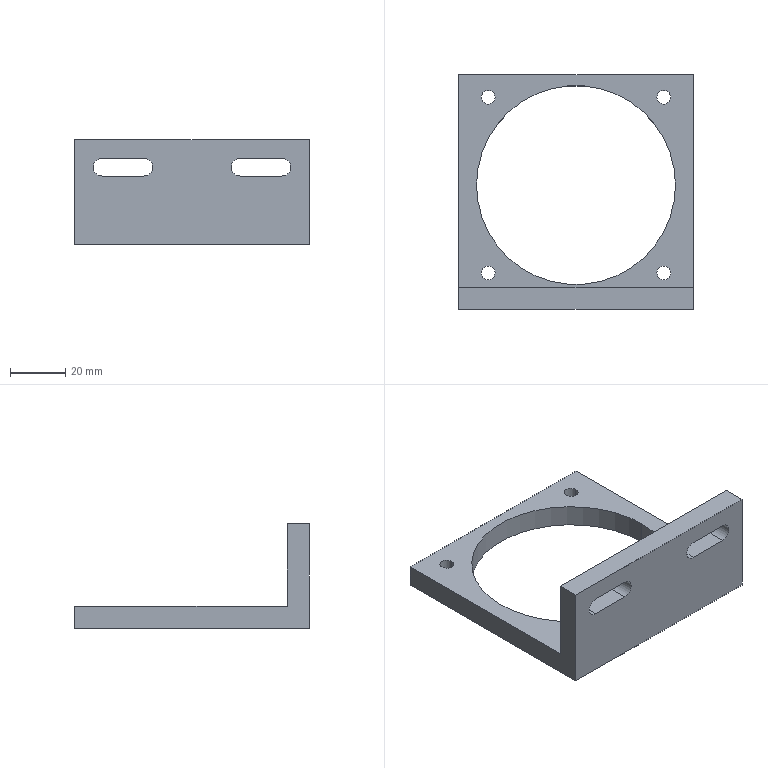Part | SolidWorks | features ICE 2, 3DProfileFeature 1, Extrusion 1, HoleWzd 1 | 1 solid | 26 faces | box 85 x 85 x 38 mm | volume 42909 mm3 | cylinder 14 | plane 12 | commonest cylinder face diameters 5 x8 6.5 x4 72 x2
STEP:
#1=CARTESIAN_POINT('',(-34.32,34.32,-4.));
#2=VERTEX_POINT('',#1);
#3=CARTESIAN_POINT('',(-29.32,34.32,-4.));
#4=VERTEX_POINT('',#3);
#5=CARTESIAN_POINT('',(-31.82,34.32,-4.));
#6=DIRECTION('',(0.,0.,1.));
#7=DIRECTION('',(1.,0.,0.));
#8=AXIS2_PLACEMENT_3D('',#5,#6,#7);
#9=CIRCLE('',#8,2.5);
#10=EDGE_CURVE('',#2,#4,#9,.T.);
#11=ORIENTED_EDGE('',*,*,#10,.F.);
#12=CARTESIAN_POINT('',(-34.32,34.32,4.));
#13=VERTEX_POINT('',#12);
#14=CARTESIAN_POINT('',(-34.32,34.32,4.));
#15=DIRECTION('',(0.,0.,1.));
#16=VECTOR('',#15,1000.);
#17=LINE('',#14,#16);
#18=EDGE_CURVE('',#2,#13,#17,.T.);
#19=ORIENTED_EDGE('',*,*,#18,.T.);
#20=CARTESIAN_POINT('',(-29.32,34.32,4.));
#21=VERTEX_POINT('',#20);
#22=CARTESIAN_POINT('',(-31.82,34.32,4.));
#23=DIRECTION('',(0.,0.,1.));
#24=DIRECTION('',(1.,0.,0.));
#25=AXIS2_PLACEMENT_3D('',#22,#23,#24);
#26=CIRCLE('',#25,2.5);
#27=EDGE_CURVE('',#13,#21,#26,.T.);
#28=ORIENTED_EDGE('',*,*,#27,.T.);
#29=CARTESIAN_POINT('',(-29.32,34.32,4.));
#30=DIRECTION('',(0.,0.,1.));
#31=VECTOR('',#30,1000.);
#32=LINE('',#29,#31);
#33=EDGE_CURVE('',#4,#21,#32,.T.);
#34=ORIENTED_EDGE('',*,*,#33,.F.);
#35=EDGE_LOOP('',(#11,#19,#28,#34));
#36=FACE_OUTER_BOUND('',#35,.T.);
#37=CARTESIAN_POINT('',(-31.82,34.32,4.));
#38=DIRECTION('',(0.,0.,1.));
#39=DIRECTION('',(1.,0.,0.));
#40=AXIS2_PLACEMENT_3D('',#37,#38,#39);
#41=CYLINDRICAL_SURFACE('',#40,2.5);
#42=ADVANCED_FACE('',(#36),#41,.F.);
#43=CARTESIAN_POINT('',(29.32,-29.32,-4.));
#44=VERTEX_POINT('',#43);
#45=CARTESIAN_POINT('',(34.32,-29.32,-4.));
#46=VERTEX_POINT('',#45);
#47=CARTESIAN_POINT('',(31.82,-29.32,-4.));
#48=DIRECTION('',(0.,0.,1.));
#49=DIRECTION('',(1.,0.,0.));
#50=AXIS2_PLACEMENT_3D('',#47,#48,#49);
#51=CIRCLE('',#50,2.5);
#52=EDGE_CURVE('',#44,#46,#51,.T.);
#53=ORIENTED_EDGE('',*,*,#52,.F.);
#54=CARTESIAN_POINT('',(29.32,-29.32,4.));
#55=VERTEX_POINT('',#54);
#56=CARTESIAN_POINT('',(29.32,-29.32,4.));
#57=DIRECTION('',(0.,0.,1.));
#58=VECTOR('',#57,1000.);
#59=LINE('',#56,#58);
#60=EDGE_CURVE('',#44,#55,#59,.T.);
#61=ORIENTED_EDGE('',*,*,#60,.T.);
#62=CARTESIAN_POINT('',(34.32,-29.32,4.));
#63=VERTEX_POINT('',#62);
#64=CARTESIAN_POINT('',(31.82,-29.32,4.));
#65=DIRECTION('',(0.,0.,1.));
#66=DIRECTION('',(1.,0.,0.));
#67=AXIS2_PLACEMENT_3D('',#64,#65,#66);
#68=CIRCLE('',#67,2.5);
#69=EDGE_CURVE('',#55,#63,#68,.T.);
#70=ORIENTED_EDGE('',*,*,#69,.T.);
#71=CARTESIAN_POINT('',(34.32,-29.32,4.));
#72=DIRECTION('',(0.,0.,1.));
#73=VECTOR('',#72,1000.);
#74=LINE('',#71,#73);
#75=EDGE_CURVE('',#46,#63,#74,.T.);
#76=ORIENTED_EDGE('',*,*,#75,.F.);
#77=EDGE_LOOP('',(#53,#61,#70,#76));
#78=FACE_OUTER_BOUND('',#77,.T.);
#79=CARTESIAN_POINT('',(31.82,-29.32,4.));
#80=DIRECTION('',(0.,0.,1.));
#81=DIRECTION('',(1.,0.,0.));
#82=AXIS2_PLACEMENT_3D('',#79,#80,#81);
#83=CYLINDRICAL_SURFACE('',#82,2.5);
#84=ADVANCED_FACE('',(#78),#83,.F.);
#85=CARTESIAN_POINT('',(-34.32,-29.32,-4.));
#86=VERTEX_POINT('',#85);
#87=CARTESIAN_POINT('',(-29.32,-29.32,-4.));
#88=VERTEX_POINT('',#87);
#89=CARTESIAN_POINT('',(-31.82,-29.32,-4.));
#90=DIRECTION('',(0.,0.,1.));
#91=DIRECTION('',(1.,0.,0.));
#92=AXIS2_PLACEMENT_3D('',#89,#90,#91);
#93=CIRCLE('',#92,2.5);
#94=EDGE_CURVE('',#86,#88,#93,.T.);
#95=ORIENTED_EDGE('',*,*,#94,.F.);
#96=CARTESIAN_POINT('',(-34.32,-29.32,4.));
#97=VERTEX_POINT('',#96);
#98=CARTESIAN_POINT('',(-34.32,-29.32,4.));
#99=DIRECTION('',(0.,0.,1.));
#100=VECTOR('',#99,1000.);
#101=LINE('',#98,#100);
#102=EDGE_CURVE('',#86,#97,#101,.T.);
#103=ORIENTED_EDGE('',*,*,#102,.T.);
#104=CARTESIAN_POINT('',(-29.32,-29.32,4.));
#105=VERTEX_POINT('',#104);
#106=CARTESIAN_POINT('',(-31.82,-29.32,4.));
#107=DIRECTION('',(0.,0.,1.));
#108=DIRECTION('',(1.,0.,0.));
#109=AXIS2_PLACEMENT_3D('',#106,#107,#108);
#110=CIRCLE('',#109,2.5);
#111=EDGE_CURVE('',#97,#105,#110,.T.);
#112=ORIENTED_EDGE('',*,*,#111,.T.);
#113=CARTESIAN_POINT('',(-29.32,-29.32,4.));
#114=DIRECTION('',(0.,0.,1.));
#115=VECTOR('',#114,1000.);
#116=LINE('',#113,#115);
#117=EDGE_CURVE('',#88,#105,#116,.T.);
#118=ORIENTED_EDGE('',*,*,#117,.F.);
#119=EDGE_LOOP('',(#95,#103,#112,#118));
#120=FACE_OUTER_BOUND('',#119,.T.);
#121=CARTESIAN_POINT('',(-31.82,-29.32,4.));
#122=DIRECTION('',(0.,0.,1.));
#123=DIRECTION('',(1.,0.,0.));
#124=AXIS2_PLACEMENT_3D('',#121,#122,#123);
#125=CYLINDRICAL_SURFACE('',#124,2.5);
#126=ADVANCED_FACE('',(#120),#125,.F.);
#127=CARTESIAN_POINT('',(29.32,34.32,-4.));
#128=VERTEX_POINT('',#127);
#129=CARTESIAN_POINT('',(34.32,34.32,-4.));
#130=VERTEX_POINT('',#129);
#131=CARTESIAN_POINT('',(31.82,34.32,-4.));
#132=DIRECTION('',(0.,0.,1.));
#133=DIRECTION('',(1.,0.,0.));
#134=AXIS2_PLACEMENT_3D('',#131,#132,#133);
#135=CIRCLE('',#134,2.5);
#136=EDGE_CURVE('',#128,#130,#135,.T.);
#137=ORIENTED_EDGE('',*,*,#136,.F.);
#138=CARTESIAN_POINT('',(29.32,34.32,4.));
#139=VERTEX_POINT('',#138);
#140=CARTESIAN_POINT('',(29.32,34.32,4.));
#141=DIRECTION('',(0.,0.,1.));
#142=VECTOR('',#141,1000.);
#143=LINE('',#140,#142);
#144=EDGE_CURVE('',#128,#139,#143,.T.);
#145=ORIENTED_EDGE('',*,*,#144,.T.);
#146=CARTESIAN_POINT('',(34.32,34.32,4.));
#147=VERTEX_POINT('',#146);
#148=CARTESIAN_POINT('',(31.82,34.32,4.));
#149=DIRECTION('',(0.,0.,1.));
#150=DIRECTION('',(1.,0.,0.));
#151=AXIS2_PLACEMENT_3D('',#148,#149,#150);
#152=CIRCLE('',#151,2.5);
#153=EDGE_CURVE('',#139,#147,#152,.T.);
#154=ORIENTED_EDGE('',*,*,#153,.T.);
#155=CARTESIAN_POINT('',(34.32,34.32,4.));
#156=DIRECTION('',(0.,0.,1.));
#157=VECTOR('',#156,1000.);
#158=LINE('',#155,#157);
#159=EDGE_CURVE('',#130,#147,#158,.T.);
#160=ORIENTED_EDGE('',*,*,#159,.F.);
#161=EDGE_LOOP('',(#137,#145,#154,#160));
#162=FACE_OUTER_BOUND('',#161,.T.);
#163=CARTESIAN_POINT('',(31.82,34.32,4.));
#164=DIRECTION('',(0.,0.,1.));
#165=DIRECTION('',(1.,0.,0.));
#166=AXIS2_PLACEMENT_3D('',#163,#164,#165);
#167=CYLINDRICAL_SURFACE('',#166,2.5);
#168=ADVANCED_FACE('',(#162),#167,.F.);
#169=CARTESIAN_POINT('',(-36.,2.5,4.));
#170=VERTEX_POINT('',#169);
#171=CARTESIAN_POINT('',(36.,2.5,4.));
#172=VERTEX_POINT('',#171);
#173=CARTESIAN_POINT('',(0.,2.5,4.));
#174=DIRECTION('',(0.,0.,1.));
#175=DIRECTION('',(1.,0.,0.));
#176=AXIS2_PLACEMENT_3D('',#173,#174,#175);
#177=CIRCLE('',#176,36.);
#178=EDGE_CURVE('',#170,#172,#177,.T.);
#179=ORIENTED_EDGE('',*,*,#178,.T.);
#180=CARTESIAN_POINT('',(36.,2.5,-4.));
#181=VERTEX_POINT('',#180);
#182=CARTESIAN_POINT('',(36.,2.5,4.));
#183=DIRECTION('',(0.,0.,-1.));
#184=VECTOR('',#183,1000.);
#185=LINE('',#182,#184);
#186=EDGE_CURVE('',#172,#181,#185,.T.);
#187=ORIENTED_EDGE('',*,*,#186,.T.);
#188=CARTESIAN_POINT('',(-36.,2.5,-4.));
#189=VERTEX_POINT('',#188);
#190=CARTESIAN_POINT('',(0.,2.5,-4.));
#191=DIRECTION('',(0.,0.,1.));
#192=DIRECTION('',(1.,0.,0.));
#193=AXIS2_PLACEMENT_3D('',#190,#191,#192);
#194=CIRCLE('',#193,36.);
#195=EDGE_CURVE('',#189,#181,#194,.T.);
#196=ORIENTED_EDGE('',*,*,#195,.F.);
#197=CARTESIAN_POINT('',(-36.,2.5,4.));
#198=DIRECTION('',(0.,0.,-1.));
#199=VECTOR('',#198,1000.);
#200=LINE('',#197,#199);
#201=EDGE_CURVE('',#170,#189,#200,.T.);
#202=ORIENTED_EDGE('',*,*,#201,.F.);
#203=EDGE_LOOP('',(#179,#187,#196,#202));
#204=FACE_OUTER_BOUND('',#203,.T.);
#205=CARTESIAN_POINT('',(0.,2.5,4.));
#206=DIRECTION('',(0.,0.,-1.));
#207=DIRECTION('',(-1.,0.,0.));
#208=AXIS2_PLACEMENT_3D('',#205,#206,#207);
#209=CYLINDRICAL_SURFACE('',#208,36.);
#210=ADVANCED_FACE('',(#204),#209,.F.);
#211=CARTESIAN_POINT('',(42.5,-34.5,4.));
#212=VERTEX_POINT('',#211);
#213=CARTESIAN_POINT('',(-42.5,-34.5,4.));
#214=VERTEX_POINT('',#213);
#215=CARTESIAN_POINT('',(-42.5,-34.5,4.));
#216=DIRECTION('',(-1.,0.,0.));
#217=VECTOR('',#216,1000.);
#218=LINE('',#215,#217);
#219=EDGE_CURVE('',#212,#214,#218,.T.);
#220=ORIENTED_EDGE('',*,*,#219,.F.);
#221=CARTESIAN_POINT('',(42.5,42.5,4.));
#222=VERTEX_POINT('',#221);
#223=CARTESIAN_POINT('',(42.5,42.5,4.));
#224=DIRECTION('',(0.,1.,0.));
#225=VECTOR('',#224,1000.);
#226=LINE('',#223,#225);
#227=EDGE_CURVE('',#212,#222,#226,.T.);
#228=ORIENTED_EDGE('',*,*,#227,.T.);
#229=CARTESIAN_POINT('',(-42.5,42.5,4.));
#230=VERTEX_POINT('',#229);
#231=CARTESIAN_POINT('',(-42.5,42.5,4.));
#232=DIRECTION('',(-1.,0.,0.));
#233=VECTOR('',#232,1000.);
#234=LINE('',#231,#233);
#235=EDGE_CURVE('',#222,#230,#234,.T.);
#236=ORIENTED_EDGE('',*,*,#235,.T.);
#237=CARTESIAN_POINT('',(-42.5,42.5,4.));
#238=DIRECTION('',(0.,-1.,0.));
#239=VECTOR('',#238,1000.);
#240=LINE('',#237,#239);
#241=EDGE_CURVE('',#230,#214,#240,.T.);
#242=ORIENTED_EDGE('',*,*,#241,.T.);
#243=EDGE_LOOP('',(#220,#228,#236,#242));
#244=FACE_OUTER_BOUND('',#243,.T.);
#245=CARTESIAN_POINT('',(-31.82,34.32,4.));
#246=DIRECTION('',(0.,0.,1.));
#247=DIRECTION('',(1.,0.,0.));
#248=AXIS2_PLACEMENT_3D('',#245,#246,#247);
#249=CIRCLE('',#248,2.5);
#250=EDGE_CURVE('',#21,#13,#249,.T.);
#251=ORIENTED_EDGE('',*,*,#250,.F.);
#252=ORIENTED_EDGE('',*,*,#27,.F.);
#253=EDGE_LOOP('',(#251,#252));
#254=FACE_BOUND('',#253,.T.);
#255=CARTESIAN_POINT('',(31.82,-29.32,4.));
#256=DIRECTION('',(0.,0.,1.));
#257=DIRECTION('',(1.,0.,0.));
#258=AXIS2_PLACEMENT_3D('',#255,#256,#257);
#259=CIRCLE('',#258,2.5);
#260=EDGE_CURVE('',#63,#55,#259,.T.);
#261=ORIENTED_EDGE('',*,*,#260,.F.);
#262=ORIENTED_EDGE('',*,*,#69,.F.);
#263=EDGE_LOOP('',(#261,#262));
#264=FACE_BOUND('',#263,.T.);
#265=CARTESIAN_POINT('',(-31.82,-29.32,4.));
#266=DIRECTION('',(0.,0.,1.));
#267=DIRECTION('',(1.,0.,0.));
#268=AXIS2_PLACEMENT_3D('',#265,#266,#267);
#269=CIRCLE('',#268,2.5);
#270=EDGE_CURVE('',#105,#97,#269,.T.);
#271=ORIENTED_EDGE('',*,*,#270,.F.);
#272=ORIENTED_EDGE('',*,*,#111,.F.);
#273=EDGE_LOOP('',(#271,#272));
#274=FACE_BOUND('',#273,.T.);
#275=CARTESIAN_POINT('',(31.82,34.32,4.));
#276=DIRECTION('',(0.,0.,1.));
#277=DIRECTION('',(1.,0.,0.));
#278=AXIS2_PLACEMENT_3D('',#275,#276,#277);
#279=CIRCLE('',#278,2.5);
#280=EDGE_CURVE('',#147,#139,#279,.T.);
#281=ORIENTED_EDGE('',*,*,#280,.F.);
#282=ORIENTED_EDGE('',*,*,#153,.F.);
#283=EDGE_LOOP('',(#281,#282));
#284=FACE_BOUND('',#283,.T.);
#285=ORIENTED_EDGE('',*,*,#178,.F.);
#286=CARTESIAN_POINT('',(0.,2.5,4.));
#287=DIRECTION('',(0.,0.,1.));
#288=DIRECTION('',(1.,0.,0.));
#289=AXIS2_PLACEMENT_3D('',#286,#287,#288);
#290=CIRCLE('',#289,36.);
#291=EDGE_CURVE('',#172,#170,#290,.T.);
#292=ORIENTED_EDGE('',*,*,#291,.F.);
#293=EDGE_LOOP('',(#285,#292));
#294=FACE_BOUND('',#293,.T.);
#295=CARTESIAN_POINT('',(0.,0.,4.));
#296=DIRECTION('',(0.,0.,1.));
#297=DIRECTION('',(1.,0.,0.));
#298=AXIS2_PLACEMENT_3D('',#295,#296,#297);
#299=PLANE('',#298);
#300=ADVANCED_FACE('',(#244,#254,#264,#274,#284,#294),#299,.T.);
#301=CARTESIAN_POINT('',(-31.82,34.32,-4.));
#302=DIRECTION('',(0.,0.,1.));
#303=DIRECTION('',(1.,0.,0.));
#304=AXIS2_PLACEMENT_3D('',#301,#302,#303);
#305=CIRCLE('',#304,2.5);
#306=EDGE_CURVE('',#4,#2,#305,.T.);
#307=ORIENTED_EDGE('',*,*,#306,.T.);
#308=ORIENTED_EDGE('',*,*,#10,.T.);
#309=EDGE_LOOP('',(#307,#308));
#310=FACE_BOUND('',#309,.T.);
#311=CARTESIAN_POINT('',(31.82,-29.32,-4.));
#312=DIRECTION('',(0.,0.,1.));
#313=DIRECTION('',(1.,0.,0.));
#314=AXIS2_PLACEMENT_3D('',#311,#312,#313);
#315=CIRCLE('',#314,2.5);
#316=EDGE_CURVE('',#46,#44,#315,.T.);
#317=ORIENTED_EDGE('',*,*,#316,.T.);
#318=ORIENTED_EDGE('',*,*,#52,.T.);
#319=EDGE_LOOP('',(#317,#318));
#320=FACE_BOUND('',#319,.T.);
#321=CARTESIAN_POINT('',(-31.82,-29.32,-4.));
#322=DIRECTION('',(0.,0.,1.));
#323=DIRECTION('',(1.,0.,0.));
#324=AXIS2_PLACEMENT_3D('',#321,#322,#323);
#325=CIRCLE('',#324,2.5);
#326=EDGE_CURVE('',#88,#86,#325,.T.);
#327=ORIENTED_EDGE('',*,*,#326,.T.);
#328=ORIENTED_EDGE('',*,*,#94,.T.);
#329=EDGE_LOOP('',(#327,#328));
#330=FACE_BOUND('',#329,.T.);
#331=CARTESIAN_POINT('',(31.82,34.32,-4.));
#332=DIRECTION('',(0.,0.,1.));
#333=DIRECTION('',(1.,0.,0.));
#334=AXIS2_PLACEMENT_3D('',#331,#332,#333);
#335=CIRCLE('',#334,2.5);
#336=EDGE_CURVE('',#130,#128,#335,.T.);
#337=ORIENTED_EDGE('',*,*,#336,.T.);
#338=ORIENTED_EDGE('',*,*,#136,.T.);
#339=EDGE_LOOP('',(#337,#338));
#340=FACE_BOUND('',#339,.T.);
#341=CARTESIAN_POINT('',(42.5,-42.5,-4.));
#342=VERTEX_POINT('',#341);
#343=CARTESIAN_POINT('',(42.5,42.5,-4.));
#344=VERTEX_POINT('',#343);
#345=CARTESIAN_POINT('',(42.5,42.5,-4.));
#346=DIRECTION('',(0.,1.,0.));
#347=VECTOR('',#346,1000.);
#348=LINE('',#345,#347);
#349=EDGE_CURVE('',#342,#344,#348,.T.);
#350=ORIENTED_EDGE('',*,*,#349,.F.);
#351=CARTESIAN_POINT('',(-42.5,-42.5,-4.));
#352=VERTEX_POINT('',#351);
#353=CARTESIAN_POINT('',(-42.5,-42.5,-4.));
#354=DIRECTION('',(1.,0.,0.));
#355=VECTOR('',#354,1000.);
#356=LINE('',#353,#355);
#357=EDGE_CURVE('',#352,#342,#356,.T.);
#358=ORIENTED_EDGE('',*,*,#357,.F.);
#359=CARTESIAN_POINT('',(-42.5,42.5,-4.));
#360=VERTEX_POINT('',#359);
#361=CARTESIAN_POINT('',(-42.5,42.5,-4.));
#362=DIRECTION('',(0.,-1.,0.));
#363=VECTOR('',#362,1000.);
#364=LINE('',#361,#363);
#365=EDGE_CURVE('',#360,#352,#364,.T.);
#366=ORIENTED_EDGE('',*,*,#365,.F.);
#367=CARTESIAN_POINT('',(-42.5,42.5,-4.));
#368=DIRECTION('',(-1.,0.,0.));
#369=VECTOR('',#368,1000.);
#370=LINE('',#367,#369);
#371=EDGE_CURVE('',#344,#360,#370,.T.);
#372=ORIENTED_EDGE('',*,*,#371,.F.);
#373=EDGE_LOOP('',(#350,#358,#366,#372));
#374=FACE_OUTER_BOUND('',#373,.T.);
#375=ORIENTED_EDGE('',*,*,#195,.T.);
#376=CARTESIAN_POINT('',(0.,2.5,-4.));
#377=DIRECTION('',(0.,0.,1.));
#378=DIRECTION('',(1.,0.,0.));
#379=AXIS2_PLACEMENT_3D('',#376,#377,#378);
#380=CIRCLE('',#379,36.);
#381=EDGE_CURVE('',#181,#189,#380,.T.);
#382=ORIENTED_EDGE('',*,*,#381,.T.);
#383=EDGE_LOOP('',(#375,#382));
#384=FACE_BOUND('',#383,.T.);
#385=CARTESIAN_POINT('',(0.,0.,-4.));
#386=DIRECTION('',(0.,0.,1.));
#387=DIRECTION('',(1.,0.,0.));
#388=AXIS2_PLACEMENT_3D('',#385,#386,#387);
#389=PLANE('',#388);
#390=ADVANCED_FACE('',(#310,#320,#330,#340,#374,#384),#389,.F.);
#391=ORIENTED_EDGE('',*,*,#349,.T.);
#392=CARTESIAN_POINT('',(42.5,42.5,4.));
#393=DIRECTION('',(0.,0.,-1.));
#394=VECTOR('',#393,1000.);
#395=LINE('',#392,#394);
#396=EDGE_CURVE('',#222,#344,#395,.T.);
#397=ORIENTED_EDGE('',*,*,#396,.F.);
#398=ORIENTED_EDGE('',*,*,#227,.F.);
#399=CARTESIAN_POINT('',(42.5,-34.5,34.));
#400=VERTEX_POINT('',#399);
#401=CARTESIAN_POINT('',(42.5,-34.5,34.));
#402=DIRECTION('',(0.,0.,-1.));
#403=VECTOR('',#402,1000.);
#404=LINE('',#401,#403);
#405=EDGE_CURVE('',#400,#212,#404,.T.);
#406=ORIENTED_EDGE('',*,*,#405,.F.);
#407=CARTESIAN_POINT('',(42.5,-42.5,34.));
#408=VERTEX_POINT('',#407);
#409=CARTESIAN_POINT('',(42.5,-42.5,34.));
#410=DIRECTION('',(0.,1.,0.));
#411=VECTOR('',#410,1000.);
#412=LINE('',#409,#411);
#413=EDGE_CURVE('',#408,#400,#412,.T.);
#414=ORIENTED_EDGE('',*,*,#413,.F.);
#415=CARTESIAN_POINT('',(42.5,-42.5,4.));
#416=DIRECTION('',(0.,0.,-1.));
#417=VECTOR('',#416,1000.);
#418=LINE('',#415,#417);
#419=EDGE_CURVE('',#408,#342,#418,.T.);
#420=ORIENTED_EDGE('',*,*,#419,.T.);
#421=EDGE_LOOP('',(#391,#397,#398,#406,#414,#420));
#422=FACE_OUTER_BOUND('',#421,.T.);
#423=CARTESIAN_POINT('',(42.5,42.5,4.));
#424=DIRECTION('',(-1.,0.,0.));
#425=DIRECTION('',(0.,-1.,0.));
#426=AXIS2_PLACEMENT_3D('',#423,#424,#425);
#427=PLANE('',#426);
#428=ADVANCED_FACE('',(#422),#427,.F.);
#429=ORIENTED_EDGE('',*,*,#371,.T.);
#430=CARTESIAN_POINT('',(-42.5,42.5,4.));
#431=DIRECTION('',(0.,0.,-1.));
#432=VECTOR('',#431,1000.);
#433=LINE('',#430,#432);
#434=EDGE_CURVE('',#230,#360,#433,.T.);
#435=ORIENTED_EDGE('',*,*,#434,.F.);
#436=ORIENTED_EDGE('',*,*,#235,.F.);
#437=ORIENTED_EDGE('',*,*,#396,.T.);
#438=EDGE_LOOP('',(#429,#435,#436,#437));
#439=FACE_OUTER_BOUND('',#438,.T.);
#440=CARTESIAN_POINT('',(-42.5,42.5,4.));
#441=DIRECTION('',(0.,-1.,0.));
#442=DIRECTION('',(0.,0.,-1.));
#443=AXIS2_PLACEMENT_3D('',#440,#441,#442);
#444=PLANE('',#443);
#445=ADVANCED_FACE('',(#439),#444,.F.);
#446=ORIENTED_EDGE('',*,*,#365,.T.);
#447=CARTESIAN_POINT('',(-42.5,-42.5,34.));
#448=VERTEX_POINT('',#447);
#449=CARTESIAN_POINT('',(-42.5,-42.5,4.));
#450=DIRECTION('',(0.,0.,-1.));
#451=VECTOR('',#450,1000.);
#452=LINE('',#449,#451);
#453=EDGE_CURVE('',#448,#352,#452,.T.);
#454=ORIENTED_EDGE('',*,*,#453,.F.);
#455=CARTESIAN_POINT('',(-42.5,-34.5,34.));
#456=VERTEX_POINT('',#455);
#457=CARTESIAN_POINT('',(-42.5,-42.5,34.));
#458=DIRECTION('',(0.,-1.,0.));
#459=VECTOR('',#458,1000.);
#460=LINE('',#457,#459);
#461=EDGE_CURVE('',#456,#448,#460,.T.);
#462=ORIENTED_EDGE('',*,*,#461,.F.);
#463=CARTESIAN_POINT('',(-42.5,-34.5,34.));
#464=DIRECTION('',(0.,0.,-1.));
#465=VECTOR('',#464,1000.);
#466=LINE('',#463,#465);
#467=EDGE_CURVE('',#456,#214,#466,.T.);
#468=ORIENTED_EDGE('',*,*,#467,.T.);
#469=ORIENTED_EDGE('',*,*,#241,.F.);
#470=ORIENTED_EDGE('',*,*,#434,.T.);
#471=EDGE_LOOP('',(#446,#454,#462,#468,#469,#470));
#472=FACE_OUTER_BOUND('',#471,.T.);
#473=CARTESIAN_POINT('',(-42.5,42.5,4.));
#474=DIRECTION('',(1.,0.,0.));
#475=DIRECTION('',(0.,1.,0.));
#476=AXIS2_PLACEMENT_3D('',#473,#474,#475);
#477=PLANE('',#476);
#478=ADVANCED_FACE('',(#472),#477,.F.);
#479=CARTESIAN_POINT('',(32.5,-42.5,20.75));
#480=VERTEX_POINT('',#479);
#481=CARTESIAN_POINT('',(17.5,-42.5,20.75));
#482=VERTEX_POINT('',#481);
#483=CARTESIAN_POINT('',(17.5,-42.5,20.75));
#484=DIRECTION('',(-1.,0.,0.));
#485=VECTOR('',#484,1000.);
#486=LINE('',#483,#485);
#487=EDGE_CURVE('',#480,#482,#486,.T.);
#488=ORIENTED_EDGE('',*,*,#487,.T.);
#489=CARTESIAN_POINT('',(17.5,-42.5,27.25));
#490=VERTEX_POINT('',#489);
#491=CARTESIAN_POINT('',(17.5,-42.5,24.));
#492=DIRECTION('',(0.,1.,0.));
#493=DIRECTION('',(0.,0.,1.));
#494=AXIS2_PLACEMENT_3D('',#491,#492,#493);
#495=CIRCLE('',#494,3.25);
#496=EDGE_CURVE('',#482,#490,#495,.T.);
#497=ORIENTED_EDGE('',*,*,#496,.T.);
#498=CARTESIAN_POINT('',(32.5,-42.5,27.25));
#499=VERTEX_POINT('',#498);
#500=CARTESIAN_POINT('',(17.5,-42.5,27.25));
#501=DIRECTION('',(1.,0.,0.));
#502=VECTOR('',#501,1000.);
#503=LINE('',#500,#502);
#504=EDGE_CURVE('',#490,#499,#503,.T.);
#505=ORIENTED_EDGE('',*,*,#504,.T.);
#506=CARTESIAN_POINT('',(32.5,-42.5,24.));
#507=DIRECTION('',(0.,1.,0.));
#508=DIRECTION('',(0.,0.,1.));
#509=AXIS2_PLACEMENT_3D('',#506,#507,#508);
#510=CIRCLE('',#509,3.25);
#511=EDGE_CURVE('',#499,#480,#510,.T.);
#512=ORIENTED_EDGE('',*,*,#511,.T.);
#513=EDGE_LOOP('',(#488,#497,#505,#512));
#514=FACE_BOUND('',#513,.T.);
#515=CARTESIAN_POINT('',(-17.5,-42.5,20.75));
#516=VERTEX_POINT('',#515);
#517=CARTESIAN_POINT('',(-32.5,-42.5,20.75));
#518=VERTEX_POINT('',#517);
#519=CARTESIAN_POINT('',(-32.5,-42.5,20.75));
#520=DIRECTION('',(-1.,0.,0.));
#521=VECTOR('',#520,1000.);
#522=LINE('',#519,#521);
#523=EDGE_CURVE('',#516,#518,#522,.T.);
#524=ORIENTED_EDGE('',*,*,#523,.T.);
#525=CARTESIAN_POINT('',(-32.5,-42.5,27.25));
#526=VERTEX_POINT('',#525);
#527=CARTESIAN_POINT('',(-32.5,-42.5,24.));
#528=DIRECTION('',(0.,1.,0.));
#529=DIRECTION('',(0.,0.,1.));
#530=AXIS2_PLACEMENT_3D('',#527,#528,#529);
#531=CIRCLE('',#530,3.25);
#532=EDGE_CURVE('',#518,#526,#531,.T.);
#533=ORIENTED_EDGE('',*,*,#532,.T.);
#534=CARTESIAN_POINT('',(-17.5,-42.5,27.25));
#535=VERTEX_POINT('',#534);
#536=CARTESIAN_POINT('',(-32.5,-42.5,27.25));
#537=DIRECTION('',(1.,0.,0.));
#538=VECTOR('',#537,1000.);
#539=LINE('',#536,#538);
#540=EDGE_CURVE('',#526,#535,#539,.T.);
#541=ORIENTED_EDGE('',*,*,#540,.T.);
#542=CARTESIAN_POINT('',(-17.5,-42.5,24.));
#543=DIRECTION('',(0.,1.,0.));
#544=DIRECTION('',(0.,0.,1.));
#545=AXIS2_PLACEMENT_3D('',#542,#543,#544);
#546=CIRCLE('',#545,3.25);
#547=EDGE_CURVE('',#535,#516,#546,.T.);
#548=ORIENTED_EDGE('',*,*,#547,.T.);
#549=EDGE_LOOP('',(#524,#533,#541,#548));
#550=FACE_BOUND('',#549,.T.);
#551=ORIENTED_EDGE('',*,*,#357,.T.);
#552=ORIENTED_EDGE('',*,*,#419,.F.);
#553=CARTESIAN_POINT('',(-42.5,-42.5,34.));
#554=DIRECTION('',(1.,0.,0.));
#555=VECTOR('',#554,1000.);
#556=LINE('',#553,#555);
#557=EDGE_CURVE('',#448,#408,#556,.T.);
#558=ORIENTED_EDGE('',*,*,#557,.F.);
#559=ORIENTED_EDGE('',*,*,#453,.T.);
#560=EDGE_LOOP('',(#551,#552,#558,#559));
#561=FACE_OUTER_BOUND('',#560,.T.);
#562=CARTESIAN_POINT('',(-42.5,-42.5,4.));
#563=DIRECTION('',(0.,1.,0.));
#564=DIRECTION('',(0.,0.,1.));
#565=AXIS2_PLACEMENT_3D('',#562,#563,#564);
#566=PLANE('',#565);
#567=ADVANCED_FACE('',(#514,#550,#561),#566,.F.);
#568=ORIENTED_EDGE('',*,*,#186,.F.);
#569=ORIENTED_EDGE('',*,*,#291,.T.);
#570=ORIENTED_EDGE('',*,*,#201,.T.);
#571=ORIENTED_EDGE('',*,*,#381,.F.);
#572=EDGE_LOOP('',(#568,#569,#570,#571));
#573=FACE_OUTER_BOUND('',#572,.T.);
#574=CARTESIAN_POINT('',(0.,2.5,4.));
#575=DIRECTION('',(0.,0.,-1.));
#576=DIRECTION('',(-1.,0.,0.));
#577=AXIS2_PLACEMENT_3D('',#574,#575,#576);
#578=CYLINDRICAL_SURFACE('',#577,36.);
#579=ADVANCED_FACE('',(#573),#578,.F.);
#580=ORIENTED_EDGE('',*,*,#144,.F.);
#581=ORIENTED_EDGE('',*,*,#336,.F.);
#582=ORIENTED_EDGE('',*,*,#159,.T.);
#583=ORIENTED_EDGE('',*,*,#280,.T.);
#584=EDGE_LOOP('',(#580,#581,#582,#583));
#585=FACE_OUTER_BOUND('',#584,.T.);
#586=CARTESIAN_POINT('',(31.82,34.32,4.));
#587=DIRECTION('',(0.,0.,1.));
#588=DIRECTION('',(1.,0.,0.));
#589=AXIS2_PLACEMENT_3D('',#586,#587,#588);
#590=CYLINDRICAL_SURFACE('',#589,2.5);
#591=ADVANCED_FACE('',(#585),#590,.F.);
#592=ORIENTED_EDGE('',*,*,#102,.F.);
#593=ORIENTED_EDGE('',*,*,#326,.F.);
#594=ORIENTED_EDGE('',*,*,#117,.T.);
#595=ORIENTED_EDGE('',*,*,#270,.T.);
#596=EDGE_LOOP('',(#592,#593,#594,#595));
#597=FACE_OUTER_BOUND('',#596,.T.);
#598=CARTESIAN_POINT('',(-31.82,-29.32,4.));
#599=DIRECTION('',(0.,0.,1.));
#600=DIRECTION('',(1.,0.,0.));
#601=AXIS2_PLACEMENT_3D('',#598,#599,#600);
#602=CYLINDRICAL_SURFACE('',#601,2.5);
#603=ADVANCED_FACE('',(#597),#602,.F.);
#604=ORIENTED_EDGE('',*,*,#60,.F.);
#605=ORIENTED_EDGE('',*,*,#316,.F.);
#606=ORIENTED_EDGE('',*,*,#75,.T.);
#607=ORIENTED_EDGE('',*,*,#260,.T.);
#608=EDGE_LOOP('',(#604,#605,#606,#607));
#609=FACE_OUTER_BOUND('',#608,.T.);
#610=CARTESIAN_POINT('',(31.82,-29.32,4.));
#611=DIRECTION('',(0.,0.,1.));
#612=DIRECTION('',(1.,0.,0.));
#613=AXIS2_PLACEMENT_3D('',#610,#611,#612);
#614=CYLINDRICAL_SURFACE('',#613,2.5);
#615=ADVANCED_FACE('',(#609),#614,.F.);
#616=ORIENTED_EDGE('',*,*,#18,.F.);
#617=ORIENTED_EDGE('',*,*,#306,.F.);
#618=ORIENTED_EDGE('',*,*,#33,.T.);
#619=ORIENTED_EDGE('',*,*,#250,.T.);
#620=EDGE_LOOP('',(#616,#617,#618,#619));
#621=FACE_OUTER_BOUND('',#620,.T.);
#622=CARTESIAN_POINT('',(-31.82,34.32,4.));
#623=DIRECTION('',(0.,0.,1.));
#624=DIRECTION('',(1.,0.,0.));
#625=AXIS2_PLACEMENT_3D('',#622,#623,#624);
#626=CYLINDRICAL_SURFACE('',#625,2.5);
#627=ADVANCED_FACE('',(#621),#626,.F.);
#628=CARTESIAN_POINT('',(17.5,-34.5,27.25));
#629=VERTEX_POINT('',#628);
#630=CARTESIAN_POINT('',(32.5,-34.5,27.25));
#631=VERTEX_POINT('',#630);
#632=CARTESIAN_POINT('',(17.5,-34.5,27.25));
#633=DIRECTION('',(1.,0.,0.));
#634=VECTOR('',#633,1000.);
#635=LINE('',#632,#634);
#636=EDGE_CURVE('',#629,#631,#635,.T.);
#637=ORIENTED_EDGE('',*,*,#636,.F.);
#638=CARTESIAN_POINT('',(17.5,-34.5,20.75));
#639=VERTEX_POINT('',#638);
#640=CARTESIAN_POINT('',(17.5,-34.5,24.));
#641=DIRECTION('',(0.,1.,0.));
#642=DIRECTION('',(0.,0.,1.));
#643=AXIS2_PLACEMENT_3D('',#640,#641,#642);
#644=CIRCLE('',#643,3.25);
#645=EDGE_CURVE('',#639,#629,#644,.T.);
#646=ORIENTED_EDGE('',*,*,#645,.F.);
#647=CARTESIAN_POINT('',(32.5,-34.5,20.75));
#648=VERTEX_POINT('',#647);
#649=CARTESIAN_POINT('',(17.5,-34.5,20.75));
#650=DIRECTION('',(-1.,0.,0.));
#651=VECTOR('',#650,1000.);
#652=LINE('',#649,#651);
#653=EDGE_CURVE('',#648,#639,#652,.T.);
#654=ORIENTED_EDGE('',*,*,#653,.F.);
#655=CARTESIAN_POINT('',(32.5,-34.5,24.));
#656=DIRECTION('',(0.,1.,0.));
#657=DIRECTION('',(0.,0.,1.));
#658=AXIS2_PLACEMENT_3D('',#655,#656,#657);
#659=CIRCLE('',#658,3.25);
#660=EDGE_CURVE('',#631,#648,#659,.T.);
#661=ORIENTED_EDGE('',*,*,#660,.F.);
#662=EDGE_LOOP('',(#637,#646,#654,#661));
#663=FACE_BOUND('',#662,.T.);
#664=CARTESIAN_POINT('',(-32.5,-34.5,27.25));
#665=VERTEX_POINT('',#664);
#666=CARTESIAN_POINT('',(-17.5,-34.5,27.25));
#667=VERTEX_POINT('',#666);
#668=CARTESIAN_POINT('',(-32.5,-34.5,27.25));
#669=DIRECTION('',(1.,0.,0.));
#670=VECTOR('',#669,1000.);
#671=LINE('',#668,#670);
#672=EDGE_CURVE('',#665,#667,#671,.T.);
#673=ORIENTED_EDGE('',*,*,#672,.F.);
#674=CARTESIAN_POINT('',(-32.5,-34.5,20.75));
#675=VERTEX_POINT('',#674);
#676=CARTESIAN_POINT('',(-32.5,-34.5,24.));
#677=DIRECTION('',(0.,1.,0.));
#678=DIRECTION('',(0.,0.,1.));
#679=AXIS2_PLACEMENT_3D('',#676,#677,#678);
#680=CIRCLE('',#679,3.25);
#681=EDGE_CURVE('',#675,#665,#680,.T.);
#682=ORIENTED_EDGE('',*,*,#681,.F.);
#683=CARTESIAN_POINT('',(-17.5,-34.5,20.75));
#684=VERTEX_POINT('',#683);
#685=CARTESIAN_POINT('',(-32.5,-34.5,20.75));
#686=DIRECTION('',(-1.,0.,0.));
#687=VECTOR('',#686,1000.);
#688=LINE('',#685,#687);
#689=EDGE_CURVE('',#684,#675,#688,.T.);
#690=ORIENTED_EDGE('',*,*,#689,.F.);
#691=CARTESIAN_POINT('',(-17.5,-34.5,24.));
#692=DIRECTION('',(0.,1.,0.));
#693=DIRECTION('',(0.,0.,1.));
#694=AXIS2_PLACEMENT_3D('',#691,#692,#693);
#695=CIRCLE('',#694,3.25);
#696=EDGE_CURVE('',#667,#684,#695,.T.);
#697=ORIENTED_EDGE('',*,*,#696,.F.);
#698=EDGE_LOOP('',(#673,#682,#690,#697));
#699=FACE_BOUND('',#698,.T.);
#700=ORIENTED_EDGE('',*,*,#219,.T.);
#701=ORIENTED_EDGE('',*,*,#467,.F.);
#702=CARTESIAN_POINT('',(-42.5,-34.5,34.));
#703=DIRECTION('',(-1.,0.,0.));
#704=VECTOR('',#703,1000.);
#705=LINE('',#702,#704);
#706=EDGE_CURVE('',#400,#456,#705,.T.);
#707=ORIENTED_EDGE('',*,*,#706,.F.);
#708=ORIENTED_EDGE('',*,*,#405,.T.);
#709=EDGE_LOOP('',(#700,#701,#707,#708));
#710=FACE_OUTER_BOUND('',#709,.T.);
#711=CARTESIAN_POINT('',(-42.5,-34.5,34.));
#712=DIRECTION('',(0.,-1.,0.));
#713=DIRECTION('',(0.,0.,-1.));
#714=AXIS2_PLACEMENT_3D('',#711,#712,#713);
#715=PLANE('',#714);
#716=ADVANCED_FACE('',(#663,#699,#710),#715,.F.);
#717=ORIENTED_EDGE('',*,*,#461,.T.);
#718=ORIENTED_EDGE('',*,*,#557,.T.);
#719=ORIENTED_EDGE('',*,*,#413,.T.);
#720=ORIENTED_EDGE('',*,*,#706,.T.);
#721=EDGE_LOOP('',(#717,#718,#719,#720));
#722=FACE_OUTER_BOUND('',#721,.T.);
#723=CARTESIAN_POINT('',(0.,0.,34.));
#724=DIRECTION('',(0.,0.,-1.));
#725=DIRECTION('',(-1.,0.,0.));
#726=AXIS2_PLACEMENT_3D('',#723,#724,#725);
#727=PLANE('',#726);
#728=ADVANCED_FACE('',(#722),#727,.F.);
#729=ORIENTED_EDGE('',*,*,#681,.T.);
#730=CARTESIAN_POINT('',(-32.5,-42.5,27.25));
#731=DIRECTION('',(0.,1.,0.));
#732=VECTOR('',#731,1000.);
#733=LINE('',#730,#732);
#734=EDGE_CURVE('',#526,#665,#733,.T.);
#735=ORIENTED_EDGE('',*,*,#734,.F.);
#736=ORIENTED_EDGE('',*,*,#532,.F.);
#737=CARTESIAN_POINT('',(-32.5,-42.5,20.75));
#738=DIRECTION('',(0.,1.,0.));
#739=VECTOR('',#738,1000.);
#740=LINE('',#737,#739);
#741=EDGE_CURVE('',#518,#675,#740,.T.);
#742=ORIENTED_EDGE('',*,*,#741,.T.);
#743=EDGE_LOOP('',(#729,#735,#736,#742));
#744=FACE_OUTER_BOUND('',#743,.T.);
#745=CARTESIAN_POINT('',(-32.5,-42.5,24.));
#746=DIRECTION('',(0.,1.,0.));
#747=DIRECTION('',(0.,0.,1.));
#748=AXIS2_PLACEMENT_3D('',#745,#746,#747);
#749=CYLINDRICAL_SURFACE('',#748,3.25);
#750=ADVANCED_FACE('',(#744),#749,.F.);
#751=ORIENTED_EDGE('',*,*,#689,.T.);
#752=ORIENTED_EDGE('',*,*,#741,.F.);
#753=ORIENTED_EDGE('',*,*,#523,.F.);
#754=CARTESIAN_POINT('',(-17.5,-42.5,20.75));
#755=DIRECTION('',(0.,1.,0.));
#756=VECTOR('',#755,1000.);
#757=LINE('',#754,#756);
#758=EDGE_CURVE('',#516,#684,#757,.T.);
#759=ORIENTED_EDGE('',*,*,#758,.T.);
#760=EDGE_LOOP('',(#751,#752,#753,#759));
#761=FACE_OUTER_BOUND('',#760,.T.);
#762=CARTESIAN_POINT('',(-32.5,-42.5,20.75));
#763=DIRECTION('',(0.,0.,-1.));
#764=DIRECTION('',(-1.,0.,0.));
#765=AXIS2_PLACEMENT_3D('',#762,#763,#764);
#766=PLANE('',#765);
#767=ADVANCED_FACE('',(#761),#766,.F.);
#768=ORIENTED_EDGE('',*,*,#696,.T.);
#769=ORIENTED_EDGE('',*,*,#758,.F.);
#770=ORIENTED_EDGE('',*,*,#547,.F.);
#771=CARTESIAN_POINT('',(-17.5,-42.5,27.25));
#772=DIRECTION('',(0.,1.,0.));
#773=VECTOR('',#772,1000.);
#774=LINE('',#771,#773);
#775=EDGE_CURVE('',#535,#667,#774,.T.);
#776=ORIENTED_EDGE('',*,*,#775,.T.);
#777=EDGE_LOOP('',(#768,#769,#770,#776));
#778=FACE_OUTER_BOUND('',#777,.T.);
#779=CARTESIAN_POINT('',(-17.5,-42.5,24.));
#780=DIRECTION('',(0.,1.,0.));
#781=DIRECTION('',(0.,0.,1.));
#782=AXIS2_PLACEMENT_3D('',#779,#780,#781);
#783=CYLINDRICAL_SURFACE('',#782,3.25);
#784=ADVANCED_FACE('',(#778),#783,.F.);
#785=ORIENTED_EDGE('',*,*,#672,.T.);
#786=ORIENTED_EDGE('',*,*,#775,.F.);
#787=ORIENTED_EDGE('',*,*,#540,.F.);
#788=ORIENTED_EDGE('',*,*,#734,.T.);
#789=EDGE_LOOP('',(#785,#786,#787,#788));
#790=FACE_OUTER_BOUND('',#789,.T.);
#791=CARTESIAN_POINT('',(-32.5,-42.5,27.25));
#792=DIRECTION('',(0.,0.,1.));
#793=DIRECTION('',(1.,0.,0.));
#794=AXIS2_PLACEMENT_3D('',#791,#792,#793);
#795=PLANE('',#794);
#796=ADVANCED_FACE('',(#790),#795,.F.);
#797=ORIENTED_EDGE('',*,*,#645,.T.);
#798=CARTESIAN_POINT('',(17.5,-42.5,27.25));
#799=DIRECTION('',(0.,1.,0.));
#800=VECTOR('',#799,1000.);
#801=LINE('',#798,#800);
#802=EDGE_CURVE('',#490,#629,#801,.T.);
#803=ORIENTED_EDGE('',*,*,#802,.F.);
#804=ORIENTED_EDGE('',*,*,#496,.F.);
#805=CARTESIAN_POINT('',(17.5,-42.5,20.75));
#806=DIRECTION('',(0.,1.,0.));
#807=VECTOR('',#806,1000.);
#808=LINE('',#805,#807);
#809=EDGE_CURVE('',#482,#639,#808,.T.);
#810=ORIENTED_EDGE('',*,*,#809,.T.);
#811=EDGE_LOOP('',(#797,#803,#804,#810));
#812=FACE_OUTER_BOUND('',#811,.T.);
#813=CARTESIAN_POINT('',(17.5,-42.5,24.));
#814=DIRECTION('',(0.,1.,0.));
#815=DIRECTION('',(0.,0.,1.));
#816=AXIS2_PLACEMENT_3D('',#813,#814,#815);
#817=CYLINDRICAL_SURFACE('',#816,3.25);
#818=ADVANCED_FACE('',(#812),#817,.F.);
#819=ORIENTED_EDGE('',*,*,#653,.T.);
#820=ORIENTED_EDGE('',*,*,#809,.F.);
#821=ORIENTED_EDGE('',*,*,#487,.F.);
#822=CARTESIAN_POINT('',(32.5,-42.5,20.75));
#823=DIRECTION('',(0.,1.,0.));
#824=VECTOR('',#823,1000.);
#825=LINE('',#822,#824);
#826=EDGE_CURVE('',#480,#648,#825,.T.);
#827=ORIENTED_EDGE('',*,*,#826,.T.);
#828=EDGE_LOOP('',(#819,#820,#821,#827));
#829=FACE_OUTER_BOUND('',#828,.T.);
#830=CARTESIAN_POINT('',(17.5,-42.5,20.75));
#831=DIRECTION('',(0.,0.,-1.));
#832=DIRECTION('',(-1.,0.,0.));
#833=AXIS2_PLACEMENT_3D('',#830,#831,#832);
#834=PLANE('',#833);
#835=ADVANCED_FACE('',(#829),#834,.F.);
#836=ORIENTED_EDGE('',*,*,#660,.T.);
#837=ORIENTED_EDGE('',*,*,#826,.F.);
#838=ORIENTED_EDGE('',*,*,#511,.F.);
#839=CARTESIAN_POINT('',(32.5,-42.5,27.25));
#840=DIRECTION('',(0.,1.,0.));
#841=VECTOR('',#840,1000.);
#842=LINE('',#839,#841);
#843=EDGE_CURVE('',#499,#631,#842,.T.);
#844=ORIENTED_EDGE('',*,*,#843,.T.);
#845=EDGE_LOOP('',(#836,#837,#838,#844));
#846=FACE_OUTER_BOUND('',#845,.T.);
#847=CARTESIAN_POINT('',(32.5,-42.5,24.));
#848=DIRECTION('',(0.,1.,0.));
#849=DIRECTION('',(0.,0.,1.));
#850=AXIS2_PLACEMENT_3D('',#847,#848,#849);
#851=CYLINDRICAL_SURFACE('',#850,3.25);
#852=ADVANCED_FACE('',(#846),#851,.F.);
#853=ORIENTED_EDGE('',*,*,#636,.T.);
#854=ORIENTED_EDGE('',*,*,#843,.F.);
#855=ORIENTED_EDGE('',*,*,#504,.F.);
#856=ORIENTED_EDGE('',*,*,#802,.T.);
#857=EDGE_LOOP('',(#853,#854,#855,#856));
#858=FACE_OUTER_BOUND('',#857,.T.);
#859=CARTESIAN_POINT('',(17.5,-42.5,27.25));
#860=DIRECTION('',(0.,0.,1.));
#861=DIRECTION('',(1.,0.,0.));
#862=AXIS2_PLACEMENT_3D('',#859,#860,#861);
#863=PLANE('',#862);
#864=ADVANCED_FACE('',(#858),#863,.F.);
#865=CLOSED_SHELL('',(#42,#84,#126,#168,#210,#300,#390,#428,#445,#478,#567,#579,#591,#603,#615,#627,#716,#728,#750,#767,#784,#796,#818,#835,#852,#864));
#866=MANIFOLD_SOLID_BREP('',#865);
#867=CARTESIAN_POINT('',(0.,0.,0.));
#868=DIRECTION('',(0.,0.,1.));
#869=DIRECTION('',(1.,0.,0.));
#870=AXIS2_PLACEMENT_3D('',#867,#868,#869);
#871=(LENGTH_UNIT()NAMED_UNIT(*)SI_UNIT(.MILLI.,.METRE.));
#872=UNCERTAINTY_MEASURE_WITH_UNIT(LENGTH_MEASURE(0.00001),#871,'','');
#873=(NAMED_UNIT(*)PLANE_ANGLE_UNIT()SI_UNIT($,.RADIAN.));
#874=(NAMED_UNIT(*)SI_UNIT($,.STERADIAN.)SOLID_ANGLE_UNIT());
#875=(GEOMETRIC_REPRESENTATION_CONTEXT(3)GLOBAL_UNCERTAINTY_ASSIGNED_CONTEXT((#872))GLOBAL_UNIT_ASSIGNED_CONTEXT((#871,#873,#874))REPRESENTATION_CONTEXT('',''));
#876=ADVANCED_BREP_SHAPE_REPRESENTATION('',(#866,#870),#875);